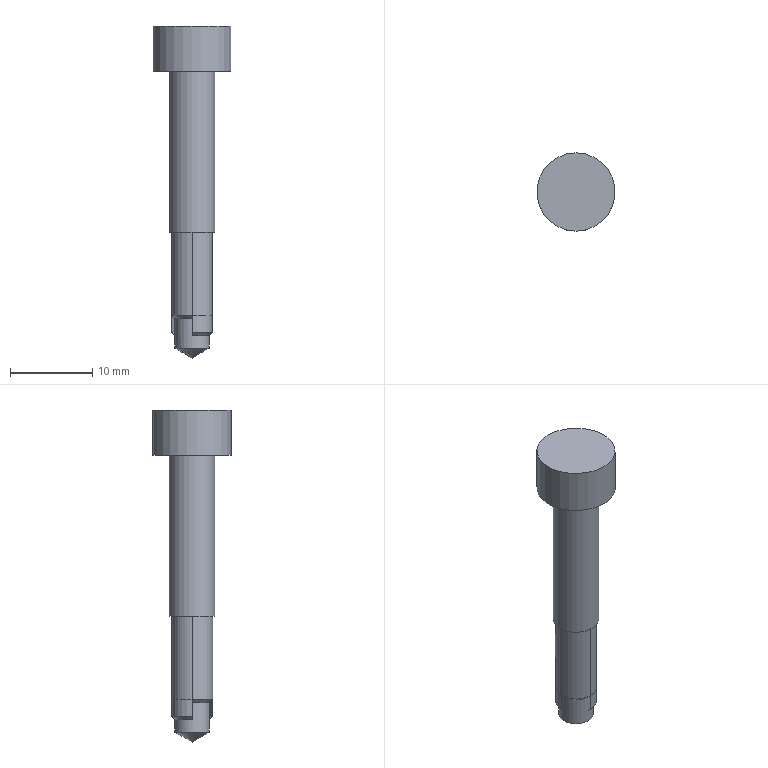Part | STEP file | EM10503000 | 3 solids | 81 faces | box 9.5 x 9.5 x 40.261 mm | volume 1873 mm3 | plane 57 | other 10 | cylinder 7 | cone 7 | commonest cylinder face diameters 5 x2 4.167 x1 4.983 x1 5.5 x1 8.5 x1 9.5 x1